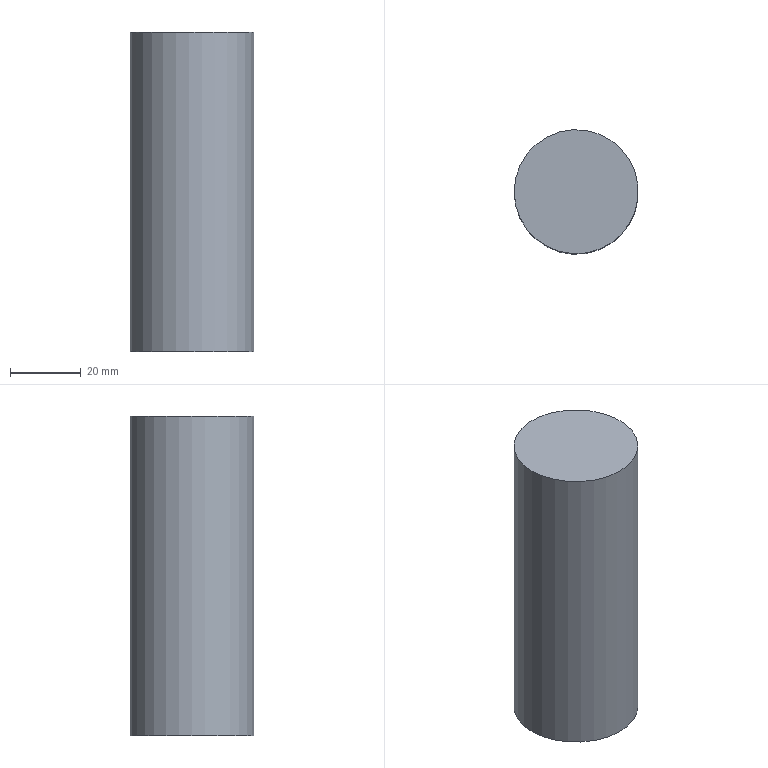Part | NX | features solid 2 | 1 solid | 3 faces | box 35 x 35 x 90 mm | volume 86590 mm3 | plane 2 | cylinder 1 | commonest cylinder face diameters 35 x1
STEP:
#1=CARTESIAN_POINT('',(-617.5,-30.,-154.));
#2=VERTEX_POINT('',#1);
#3=CARTESIAN_POINT('',(-600.,-30.,-154.));
#4=DIRECTION('',(0.,0.,-1.));
#5=DIRECTION('',(-1.,0.,0.));
#6=AXIS2_PLACEMENT_3D('',#3,#4,#5);
#7=CIRCLE('',#6,17.5);
#8=EDGE_CURVE('',#2,#2,#7,.T.);
#9=ORIENTED_EDGE('',*,*,#8,.F.);
#10=EDGE_LOOP('',(#9));
#11=FACE_BOUND('',#10,.T.);
#12=CARTESIAN_POINT('',(-617.5,-30.,-64.));
#13=VERTEX_POINT('',#12);
#14=CARTESIAN_POINT('',(-600.,-30.,-64.));
#15=DIRECTION('',(0.,0.,-1.));
#16=DIRECTION('',(-1.,0.,0.));
#17=AXIS2_PLACEMENT_3D('',#14,#15,#16);
#18=CIRCLE('',#17,17.5);
#19=EDGE_CURVE('',#13,#13,#18,.T.);
#20=ORIENTED_EDGE('',*,*,#19,.T.);
#21=EDGE_LOOP('',(#20));
#22=FACE_BOUND('',#21,.T.);
#23=CARTESIAN_POINT('',(-600.,-30.,-154.));
#24=DIRECTION('',(0.,0.,1.));
#25=DIRECTION('',(-1.,0.,0.));
#26=AXIS2_PLACEMENT_3D('',#23,#24,#25);
#27=CYLINDRICAL_SURFACE('',#26,17.5);
#28=ADVANCED_FACE('',(#11,#22),#27,.T.);
#29=ORIENTED_EDGE('',*,*,#8,.T.);
#30=EDGE_LOOP('',(#29));
#31=FACE_BOUND('',#30,.T.);
#32=CARTESIAN_POINT('',(-600.,-30.,-154.));
#33=DIRECTION('',(0.,0.,1.));
#34=DIRECTION('',(1.,0.,0.));
#35=AXIS2_PLACEMENT_3D('',#32,#33,#34);
#36=PLANE('',#35);
#37=ADVANCED_FACE('',(#31),#36,.F.);
#38=ORIENTED_EDGE('',*,*,#19,.F.);
#39=EDGE_LOOP('',(#38));
#40=FACE_BOUND('',#39,.T.);
#41=CARTESIAN_POINT('',(-600.,-30.,-64.));
#42=DIRECTION('',(0.,0.,1.));
#43=DIRECTION('',(1.,0.,0.));
#44=AXIS2_PLACEMENT_3D('',#41,#42,#43);
#45=PLANE('',#44);
#46=ADVANCED_FACE('',(#40),#45,.T.);
#47=CLOSED_SHELL('',(#28,#37,#46));
#48=MANIFOLD_SOLID_BREP('',#47);
#49=(LENGTH_UNIT()NAMED_UNIT(*)SI_UNIT(.MILLI.,.METRE.));
#50=UNCERTAINTY_MEASURE_WITH_UNIT(LENGTH_MEASURE(0.00001),#49,'','');
#51=(NAMED_UNIT(*)PLANE_ANGLE_UNIT()SI_UNIT($,.RADIAN.));
#52=(NAMED_UNIT(*)SI_UNIT($,.STERADIAN.)SOLID_ANGLE_UNIT());
#53=(GEOMETRIC_REPRESENTATION_CONTEXT(3)GLOBAL_UNCERTAINTY_ASSIGNED_CONTEXT((#50))GLOBAL_UNIT_ASSIGNED_CONTEXT((#49,#51,#52))REPRESENTATION_CONTEXT('',''));
#54=ADVANCED_BREP_SHAPE_REPRESENTATION('',(#48),#53);